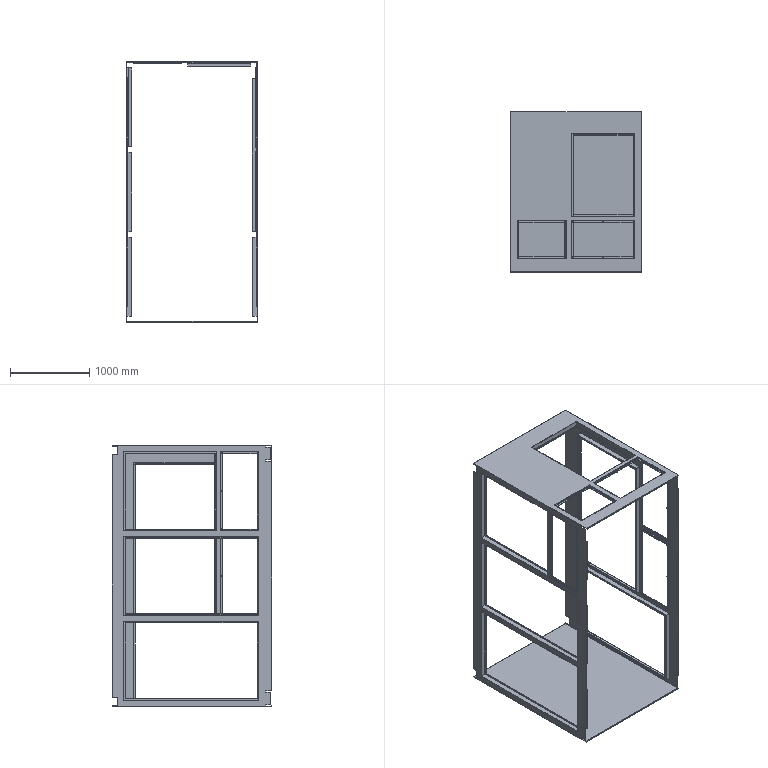Part | SolidWorks | 29 solids | 1841 faces | box 1655 x 2018 x 3305 mm | volume 30330436 mm3 | plane 1063 | cylinder 374 | cone 224 | spline 180 | commonest cylinder face diameters 5.2 x111 0.2 x110 9 x75 6.647 x56 2 x9 7 x9